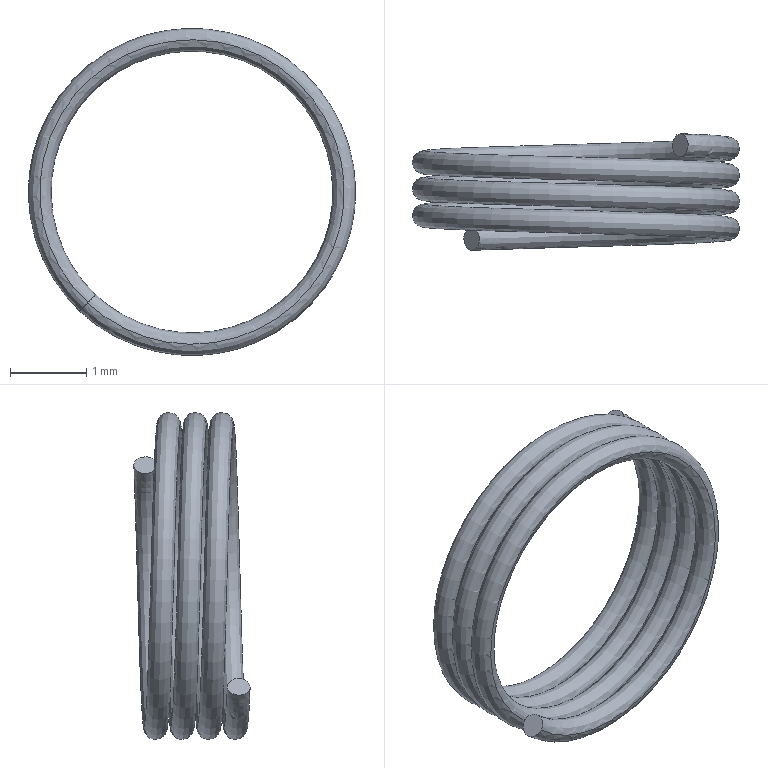Part | SolidWorks | features BaseBody 1 | 1 solid | 4 faces | box 4.301 x 1.528 x 4.3 mm | volume 3.11 mm3 | plane 2 | spline 2